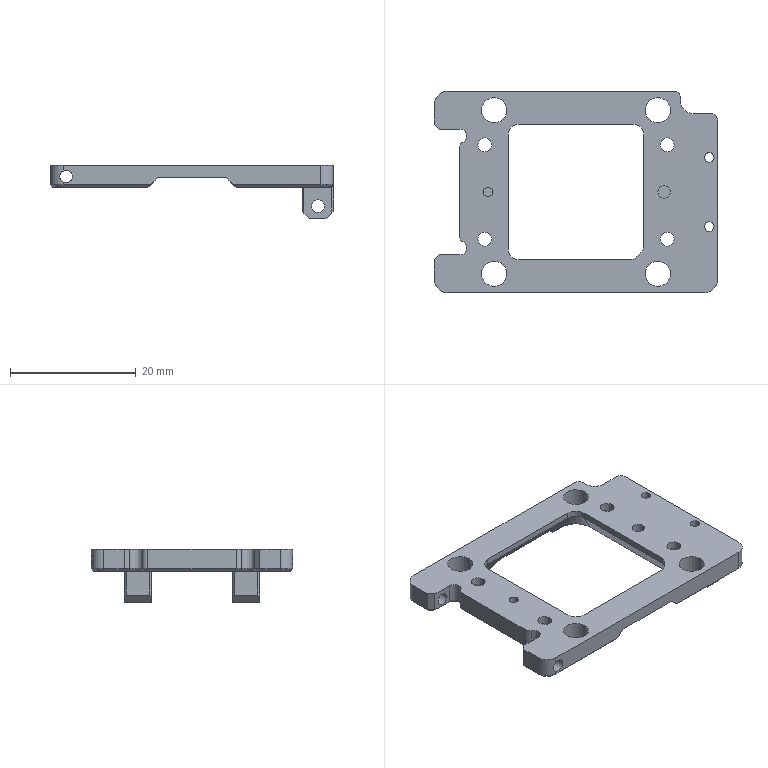NC program | NX | posted with a generic post | part box 45 x 32 x 8.5 mm
Lines 1 to 868 of 3806:
N10 G17 G21 G94 G90
(FLOOR_WALL , TOOL : D63)
N12 T03 M6
N14 G54
N16 G17 G0 G90 X-60. Y-1. B0. C0. S6500 M3
N18 G43 Z30. H3
N20 Z3.
N22 G94 G1 Z0. F1250.
N24 X-57.
N26 X57.
N28 X60.
N30 Z3.
N32 G0 Z30.
N34 M5
(DRILLING , TOOL : D6A45)
N36 T01 M6
N38 G54
N40 G17 G0 G90 X-13. Y13. B0. C0. S5000 M3
N42 G43 Z30. H1
N44 G94 G81 G98 Z-0.6 F250. R3.
N46 X-14.5 Y7.5
N48 X-14. Y0.
N50 X-14.5 Y-7.5
N52 X-13. Y-13.
N54 X13.
N56 X14.5 Y-7.5
N58 X21.2 Y-5.5
N60 X14. Y0.
N62 X21.2 Y5.5
N64 X14.5 Y7.5
N66 X13. Y13.
N68 G80
N70 G0 X13. Y13. Z30.
N72 M5
(DRILLING_COPY_COPY , TOOL : 2.2ZT)
N74 T12 M6
N76 G54
N78 G17 G0 G90 X14.5 Y7.5 B0. C0. S1447 M3
N80 G43 Z30. H12
N82 G94 G83 G98 Z-3.461 F100. Q2. R3.
N84 Y-7.5
N86 X-14.5
N88 Y7.5
N90 G80
N92 G0 X-14.5 Y7.5 Z30.
N94 M5
(DRILLING_COPY_COPY_1 , TOOL : 1.5ZT)
N96 T20 M6
N98 G54
N100 G17 G0 G90 X21.2 Y5.5 B0. C0. S2000 M3
N102 G43 Z30. H20
N104 G94 G83 G98 Z-5.451 F100. Q1. R3.
N106 Y-5.5
N108 G80
N110 G0 X21.2 Y-5.5 Z30.
N112 M5
(DRILLING_COPY_COPY_COPY , TOOL : 4.0ZT)
N114 T09 M6
N116 G54
N118 G17 G0 G90 X13. Y13. B0. C0. S1447 M3
N120 G43 Z30. H9
N122 G94 G83 G98 Z-6.202 F100. Q2. R3.
N124 Y-13.
N126 X-13.
N128 Y13.
N130 G80
N132 G0 X-13. Y13. Z30.
N134 M5
(ADAPTIVE_MILLING , TOOL : D6)
N136 T06 M6
N138 G54
N140 G17 G0 G90 X-30.144 Y-10.787 B0. C0. S9500 M3
N142 G43 Z30. H6
N144 Z-7.5
N146 G94 G1 Z-8.5 F1000.
N148 X-29.181 Y-11.11 F3000.
N150 G3 X-28.537 Y-10.787 R0.611
N152 X-28.017 Y-8.202 R6.628
N154 X-27.907 Y-0.404 R180.736
N156 G2 X-27.878 Y15.57 R931.852
N158 X-25.51 Y18.38 R3.94
N160 X-21.131 Y19.288 R11.792
N162 X-11.833 Y19.393 R240.476
N164 G1 X23.717
N166 X23.792 Y19.392
N168 X23.867 Y19.388
N170 X23.942 Y19.382
N172 X24.017 Y19.374
N174 G2 X26.858 Y17.047 R3.894
N176 X27.794 Y12.524 R11.939
N178 X27.892 Y4.2 R244.742
N180 G1 X27.893 Y-7.725
N182 Y-17.175
N184 X27.892 Y-17.25
N186 X27.89 Y-17.325
N188 X27.885 Y-17.4
N190 X27.878 Y-17.474
N192 G2 X25.646 Y-20.3 R3.826
N194 X21.282 Y-21.263 R11.208
N196 X9.584 Y-21.381 R273.049
N198 G1 X-23.716 Y-21.392
N200 X-23.791 Y-21.391
N202 X-23.866 Y-21.387
N204 X-23.94 Y-21.381
N206 X-24.015 Y-21.374
N208 G2 X-26.857 Y-19.048 R3.893
N210 X-27.79 Y-14.599 R11.787
N212 X-27.584 Y-9.889 R22.068
N214 G3 X-27.317 Y-0.896 R98.508
N216 G1 X-27.314 Y1.579
N218 X-27.312 Y9.004
N220 Y13.354
N222 X-27.309 Y13.504
N224 X-27.301 Y13.653
N226 X-27.289 Y13.803
N228 G2 X-24.364 Y17.613 R4.867
N230 G3 X-23.036 Y18.476 R5.511
N232 G2 X-20.479 Y19.15 R6.035
N234 G1 X15.597
N236 X15.639 Y19.147
N238 G3 X22.125 Y18.8 R44.001
N240 G2 X26.031 Y16.016 R4.79
N242 X27.152 Y11.077 R12.682
N244 X27.285 Y1.854 R189.651
N246 G1 X27.287 Y-6.471
N248 Y-15.321
N250 X27.285 Y-15.471
N252 X27.279 Y-15.621
N254 X27.268 Y-15.77
N256 G2 X24.43 Y-19.558 R4.81
N258 X19.706 Y-20.627 R12.635
N260 X11.159 Y-20.772 R162.134
N262 G1 X6.134 Y-20.776
N264 X-21.841 Y-20.785
N266 X-21.916
N268 X-22.066 Y-20.78
N270 X-22.141 Y-20.776
N272 X-22.291 Y-20.765
N274 G2 X-26.107 Y-17.851 R4.85
N276 X-27.075 Y-11.916 R12.339
N278 G3 X-26.72 Y3.151 R200.631
N280 G2 X-26.68 Y12.525 R294.534
N282 X-25.449 Y15.393 R5.271
N284 X-24.108 Y17.667 R5.815
N286 G1 X-23.87 Y17.85
N288 G3 X-23.636 Y18.321 R0.614
N290 G1 X-23.633 Y18.64
N292 X-23.624 Y19.84 Z-8.4
N294 G2 X-23.172 Y20.458 R0.607
N296 X-20.976 Y20.885 R12.212
N298 G1 X-19.668 Y20.971
N300 X-18.358 Y21.014
N302 X15.308 Y21.35
N304 G2 X15.898 Y20.886 R0.605
N306 G1 X15.957 Y20.634
N308 X16.227 Y19.465 Z-8.5
N310 G3 X16.658 Y19.012 R0.609
N312 X20.024 Y18.321 R9.085
N314 G2 X25.587 Y14.508 R5.788
N316 X26.57 Y9.074 R16.422
N318 X26.679 Y-0.15 R275.392
N320 G1 X26.68 Y-7.8
N322 Y-13.725
N324 X26.678 Y-13.95
N326 X26.676 Y-14.025
N328 X26.667 Y-14.25
N330 X26.656 Y-14.399
N332 G2 X23.298 Y-18.928 R5.473
N334 X18.044 Y-20.03 R14.603
N336 X8.671 Y-20.167 R206.376
N338 G1 X2.446 Y-20.171
N340 X-20.279 Y-20.178
N342 X-20.429 Y-20.176
N344 X-20.579 Y-20.172
N346 X-20.729 Y-20.166
N348 X-20.804 Y-20.162
N350 G2 X-25.394 Y-16.891 R5.458
N352 X-26.346 Y-11.925 R11.302
N354 G3 X-26.112 Y10.797 R716.655
N356 G2 X-25.65 Y13.207 R8.49
N358 X-25.43 Y15.441 R9.186
N360 G3 X-25.434 Y15.909 R0.625
N362 G1 X-25.647 Y16.399
N364 X-26.124 Y17.5 Z-8.4
N366 G2 X-26.129 Y18.049 R0.62
N368 X-25.644 Y18.838 R3.077
N370 G1 X-24.474 Y19.864
N372 G2 X-23.035 Y20.56 R4.205
N374 X-20.895 Y20.94 R13.721
N376 G1 X-19.868 Y21.027
N378 X-18.839 Y21.06
N380 X15.873 Y21.126
N382 G2 X16.487 Y20.564 R0.644
N384 G1 X16.812 Y19.409 Z-8.5
N386 X16.882 Y19.165
N388 X17.005 Y18.944
N390 X17.108 Y18.858
N392 X17.223 Y18.788
N394 G3 X18.553 Y18.184 R32.681
N396 G2 X21.165 Y17.512 R33.868
N398 X24.857 Y13.822 R6.643
N400 X25.68 Y11.433 R4.399
N402 X26.059 Y3.423 R64.029
N404 X26.038 Y-13.301 R759.858
N406 X25.37 Y-15.584 R5.874
N408 X24.108 Y-17.667 R5.525
N410 X21.791 Y-18.98 R5.884
N412 X12.51 Y-19.543 R63.462
N414 G1 X11.31 Y-19.551
N416 X9.811 Y-19.556
N418 X7.486 Y-19.561
N420 X2.161 Y-19.564
N422 X-18.914 Y-19.571
N424 X-19.139 Y-19.569
N426 G2 X-22.097 Y-18.865 R6.159
N428 X-24.167 Y-17.608 R5.507
N430 X-25.48 Y-15.291 R5.884
N432 X-25.69 Y-10.305 R26.123
N434 G3 X-25.525 Y9.942 R789.618
N436 G1 X-25.548 Y10.026
N438 X-25.647 Y10.779
N440 X-25.65 Y10.821
N442 Y13.221
N444 G3 X-26.039 Y13.786 R0.618
N446 G1 X-27.109 Y14.328 Z-8.4
N448 G2 X-27.561 Y14.757 R0.745
N450 G1 X-27.588 Y14.943
N452 X-27.559 Y15.13
N454 G2 X-26.896 Y16.878 R13.154
N456 X-25.822 Y18.586 R8.756
N458 X-22.937 Y20.573 R6.783
N460 X-20.073 Y21.13 R7.715
N462 G1 X13.95 Y21.123
N464 G2 X16.48 Y20.881 R24.277
N466 X16.878 Y20.519 R0.613
N468 G1 X17.317 Y19.403 Z-8.5
N470 X17.583 Y18.743
N472 X17.739 Y18.561
N474 G3 X19.968 Y17.353 R7.024
N476 G2 X22.834 Y15.35 R8.241
N478 X24.871 Y13.803 R4.032
N480 G3 X25.76 Y14.755 R-0.66
N482 G1 X23.431 Y16.302
N484 X22.431 Y16.966 Z-8.4
N486 X19.892 Y18.654
N488 X18.964 Y19.263 Z-8.492
N490 X18.88 Y19.297 Z-8.5
N492 G3 X18.273 Y18.147 R0.66
N494 X20.687 Y16.306 R28.606
N496 X21.736 Y15.556 R4.244
N498 G2 X22.959 Y15.286 R3.477
N500 G3 X23.756 Y16.27 R0.66
N502 X23.299 Y16.609 Z-8.452 R1.319
N504 G1 X22.759 Y16.924 Z-8.4
N506 X19.973 Y18.55
N508 X19.651 Y18.742 Z-8.431
N510 X19.316 Y18.911 Z-8.463
N512 G3 X18.877 Y18.896 Z-8.5 R0.679
N514 X18.594 Y17.885 R0.662
N516 X20.854 Y15.619 R7.438
N518 G1 X20.926 Y15.6
N520 X21.003 Y15.587
N522 X21.479
N524 X21.521 Y15.585
N526 X21.744 Y15.555
N528 G3 X22.186 Y16.765 R0.66
N530 G1 X21.037 Y17.506
N532 X19.878 Y18.232
N534 G3 X19.092 Y17.227 R0.66
N536 X19.718 Y16.163 R27.834
N538 X21.026 Y15.587 R1.251
N540 X21.417 Y16.779 R0.66
N542 G1 X20.24 Y17.636
N544 G3 X19.327 Y16.801 R0.661
N546 X19.872 Y15.742 R3.008
N548 X20.548 Y15.587 R1.151
N550 X20.839 Y16.839 R0.66
N552 G1 X20.385 Y17.054
N554 G3 X19.58 Y16.175 R0.661
N556 G1 X19.612 Y16.096
N558 X19.671 Y15.984
N560 X19.73 Y15.895
N562 X19.781 Y15.84
N564 G3 X20.116 Y15.622 R0.673
N566 G1 X20.323 Y15.587
N568 X21.521 Y15.585
N570 X22.068 Y15.518
N572 X22.613 Y15.43
N574 X23.114 Y15.227
N576 X23.608 Y15.006
N578 X24.04 Y14.68
N580 X24.46 Y14.339
N582 X24.793 Y13.912
N584 X25.11 Y13.474
N586 X25.322 Y12.976
N588 X25.514 Y12.47
N590 X25.647 Y11.458
N592 X25.65 Y11.416
N594 Y-13.979
N596 X25.647 Y-14.021
N598 X25.48 Y-15.291
N600 X25.459 Y-15.372
N602 X25.344 Y-15.649
N604 X25.148 Y-16.132
N606 X24.935 Y-16.608
N608 X24.531 Y-17.145
N610 X24.108 Y-17.667
N612 X23.58 Y-18.081
N614 X23.036 Y-18.476
N616 X22.418 Y-18.739
N618 X21.791 Y-18.98
N620 X20.521 Y-19.147
N622 X20.479 Y-19.15
N624 X-20.479
N626 X-20.521 Y-19.147
N628 X-21.791 Y-18.98
N630 X-21.872 Y-18.959
N632 X-22.149 Y-18.844
N634 X-22.632 Y-18.648
N636 X-23.108 Y-18.435
N638 X-23.645 Y-18.031
N640 X-24.167 Y-17.608
N642 X-24.581 Y-17.08
N644 X-24.976 Y-16.536
N646 X-25.239 Y-15.918
N648 X-25.48 Y-15.291
N650 X-25.65 Y-13.979
N652 Y-10.821
N654 X-25.647 Y-10.779
N656 G2 X-25.297 Y-9. R14.745
N658 G3 X-24.966 Y-2.563 R49.993
N660 G1 X-24.954 Y-1.213
N662 X-24.944 Y0.212
N664 X-24.939 Y1.637
N666 X-24.936 Y2.837
N668 X-24.933 Y3.512
N670 X-24.931 Y4.562
N672 Y5.387
N674 X-24.928 Y6.137
N676 Y6.737
N678 X-24.925 Y7.487
N680 X-24.92 Y8.237
N682 Y8.461
N684 X-24.923 Y8.611
N686 X-24.929 Y8.686
N688 X-24.943 Y8.76
N690 G3 X-25.244 Y9.264 R3.63
N692 G1 X-25.527 Y9.946
N694 G3 X-26.517 Y10.233 R0.662
N696 X-26.796 Y9.58 Z-8.438 R0.712
N698 G1 Y9.124 Z-8.4
N700 Y-9.084
N702 X-26.8 Y-9.462 Z-8.432
N704 X-26.778 Y-9.84 Z-8.463
N706 G3 X-26.549 Y-10.209 Z-8.5 R0.681
N708 X-25.527 Y-9.946 R0.662
N710 X-24.532 Y-5.98 R9.59
N712 X-24.333 Y5.191 R192.621
N714 X-24.398 Y8.112 R22.651
N716 X-24.74 Y8.589 R1.366
N718 G1 X-25.06 Y9.006
N720 G3 X-25.902 Y9.182 R0.664
N722 X-26.244 Y8.498 Z-8.433 R0.702
N724 G1 X-26.247 Y8.108 Z-8.4
N726 X-26.382 Y-8.264
N728 X-26.387 Y-8.597 Z-8.428
N730 X-26.37 Y-8.929 Z-8.456
N732 G3 X-26.071 Y-9.353 Z-8.5 R0.668
N734 X-25.203 Y-9.192 R0.664
N736 X-24.136 Y-6.512 R5.083
N738 X-23.774 Y-0.003 R48.227
N740 X-23.792 Y7.195 R108.609
N742 X-23.993 Y7.838 R1.451
N744 G1 X-24.576 Y8.421
N746 G3 X-25.367 Y8.53 R0.665
N748 X-25.705 Y7.855 Z-8.434 R0.705
N750 G1 X-25.714 Y7.453 Z-8.4
N752 X-26.055 Y-7.829
N754 X-26.065 Y-8.165 Z-8.428
N756 X-26.052 Y-8.501 Z-8.456
N758 G3 X-25.767 Y-8.926 Z-8.5 R0.669
N760 X-24.883 Y-8.775 R0.664
N762 X-23.642 Y-6.123 R4.829
N764 X-23.194 Y0.003 R37.335
N766 X-23.204 Y6.451 R93.375
N768 X-23.549 Y7.499 R1.644
N770 G1 X-23.907 Y7.758
N772 X-23.945 Y7.791
N774 X-23.998 Y7.844
N776 G3 X-24.779 Y7.958 R0.665
N778 X-25.129 Y7.288 Z-8.434 R0.705
N780 G1 X-25.145 Y6.888 Z-8.4
N782 X-25.712 Y-7.426
N784 X-25.728 Y-7.763 Z-8.428
N786 X-25.721 Y-8.101 Z-8.456
N788 G3 X-25.446 Y-8.53 Z-8.5 R0.669
N790 X-24.607 Y-8.452 R0.664
N792 X-23.156 Y-5.807 R4.552
N794 X-22.618 Y0.083 R30.621
N796 X-22.636 Y5.93 R60.554
N798 X-23.019 Y7.122 R1.986
N800 G1 X-23.077 Y7.169
N802 X-23.111 Y7.193
N804 X-23.157 Y7.216
N806 X-23.583 Y7.524
N808 G3 X-24.311 Y7.553 R0.666
N810 X-24.634 Y6.907 Z-8.437 R0.707
N812 G1 X-24.653 Y6.467 Z-8.4
N814 X-25.232 Y-6.941
N816 X-25.249 Y-7.28 Z-8.428
N818 X-25.245 Y-7.62 Z-8.457
N820 G3 X-24.975 Y-8.048 Z-8.5 R0.67
N822 X-24.129 Y-7.974 R0.664
N824 X-22.666 Y-5.498 R4.261
N826 X-22.042 Y0.307 R27.072
N828 X-22.103 Y5.701 R36.776
N830 X-22.626 Y6.995 R2.077
N832 G1 X-22.689 Y7.036
N834 X-22.766 Y7.076
N836 X-23.067 Y7.171
N838 X-23.134 Y7.205
N840 G3 X-23.774 Y7.179 R0.67
N842 X-24.097 Y6.541 Z-8.438 R0.71
N844 G1 X-24.123 Y6.092 Z-8.4
N846 X-24.86 Y-6.592
N848 X-24.885 Y-6.947 Z-8.43
N850 X-24.879 Y-7.302 Z-8.459
N852 G3 X-24.628 Y-7.707 Z-8.5 R0.672
N854 X-23.846 Y-7.714 R0.665
N856 X-22.22 Y-5.368 R3.844
N858 X-21.65 Y-2.299 R16.994
N860 X-21.681 Y5.5 R315.492
N862 X-22.216 Y6.865 R2.088
N864 G1 X-22.783 Y7.081
N866 G3 X-23.577 Y6.166 R0.661
N868 G1 X-22.853 Y4.675
N870 G3 X-21.65 Y5.051 R0.66
N872 X-21.761 Y6.535 R4.031
N874 X-22.365 Y6.948 R0.954
N876 X-23.063 Y5.887 R0.66
N878 G1 X-22.87 Y5.658
N880 X-22.646 Y5.457
N882 G3 X-21.65 Y6.026 R0.661
N884 X-21.941 Y6.753 R0.822
N886 X-22.982 Y6.29 R0.661
N888 G1 X-23.014 Y6.002
N890 X-23.149 Y4.81 Z-8.4
N892 X-24.401 Y-6.253
N894 X-24.446 Y-6.605 Z-8.43
N896 X-24.459 Y-6.959 Z-8.459
N898 G3 X-24.23 Y-7.378 Z-8.5 R0.672
N900 X-23.42 Y-7.406 R0.665
N902 X-21.77 Y-5.23 R3.687
N904 G1 X-21.721 Y-5.088
N906 X-21.674 Y-4.946
N908 X-21.657 Y-4.873
N910 X-21.65 Y-4.821
N912 Y-2.271
N914 G3 X-22.773 Y-1.8 R0.661
N916 X-22.994 Y-2.285 Z-8.455 R0.909
N918 G1 X-23.153 Y-2.924 Z-8.4
N920 X-23.894 Y-5.898
N922 X-23.985 Y-6.243 Z-8.43
N924 X-24.045 Y-6.594 Z-8.46
N926 G3 X-23.875 Y-7.037 Z-8.5 R0.673
N928 X-23.09 Y-7.182 R0.665
N930 X-21.65 Y-5.695 R2.302
N932 G1 Y-4.795
N934 G3 X-22.905 Y-4.51 R0.66
N936 G1 X-23.758 Y-6.314
N938 G3 X-22.924 Y-7.126 R0.661
N940 X-21.681 Y-6.254 R1.713
N942 G1 X-21.662 Y-6.181
N944 X-21.65 Y-6.107
N946 Y-5.657
N948 G3 X-22.869 Y-5.306 R0.66
N950 G1 X-23.374 Y-6.127
N952 G3 X-22.567 Y-7.012 R0.661
N954 X-21.69 Y-6.399 R1.092
N956 G1 X-21.66 Y-6.289
N958 X-21.65 Y-6.176
N960 Y-6.101
N962 G3 X-22.297 Y-5.497 R0.609
N964 G1 X-23.159 Y-5.555
N966 Z-5.5
N968 G0 Z30.
N970 X2.147 Y-1.637
N972 Z1.
N974 G3 X2.147 Y-1.637 Z0.763 I-2.147 J1.637 F1000.
N976 X2.147 Y-1.637 Z0.526 I-2.147 J1.637
N978 X2.147 Y-1.637 Z0.289 I-2.147 J1.637
N980 X2.147 Y-1.637 Z0.052 I-2.147 J1.637
N982 X2.147 Y-1.637 Z-0.184 I-2.147 J1.637
N984 X2.147 Y-1.637 Z-0.421 I-2.147 J1.637
N986 X2.147 Y-1.637 Z-0.658 I-2.147 J1.637
N988 X2.147 Y-1.637 Z-0.895 I-2.147 J1.637
N990 X2.147 Y-1.637 Z-1.132 I-2.147 J1.637
N992 X2.147 Y-1.637 Z-1.369 I-2.147 J1.637
N994 X2.147 Y-1.637 Z-1.606 I-2.147 J1.637
N996 X2.147 Y-1.637 Z-1.843 I-2.147 J1.637
N998 X2.147 Y-1.637 Z-2.08 I-2.147 J1.637
N1000 X2.147 Y-1.637 Z-2.316 I-2.147 J1.637
N1002 X2.147 Y-1.637 Z-2.553 I-2.147 J1.637
N1004 X2.147 Y-1.637 Z-2.79 I-2.147 J1.637
N1006 X2.147 Y-1.637 Z-3.027 I-2.147 J1.637
N1008 X2.147 Y-1.637 Z-3.264 I-2.147 J1.637
N1010 X2.147 Y-1.637 Z-3.501 I-2.147 J1.637
N1012 X2.147 Y-1.637 Z-3.738 I-2.147 J1.637
N1014 X2.147 Y-1.637 Z-3.975 I-2.147 J1.637
N1016 X2.147 Y-1.637 Z-4.211 I-2.147 J1.637
N1018 X2.147 Y-1.637 Z-4.448 I-2.147 J1.637
N1020 X2.147 Y-1.637 Z-4.685 I-2.147 J1.637
N1022 X2.147 Y-1.637 Z-4.922 I-2.147 J1.637
N1024 X2.147 Y-1.637 Z-5.159 I-2.147 J1.637
N1026 X2.147 Y-1.637 Z-5.396 I-2.147 J1.637
N1028 X2.147 Y-1.637 Z-5.633 I-2.147 J1.637
N1030 X2.147 Y-1.637 Z-5.87 I-2.147 J1.637
N1032 X2.147 Y-1.637 Z-6.107 I-2.147 J1.637
N1034 X2.147 Y-1.637 Z-6.343 I-2.147 J1.637
N1036 X2.147 Y-1.637 Z-6.58 I-2.147 J1.637
N1038 X2.147 Y-1.637 Z-6.817 I-2.147 J1.637
N1040 X2.147 Y-1.637 Z-7.054 I-2.147 J1.637
N1042 X2.147 Y-1.637 Z-7.291 I-2.147 J1.637
N1044 X2.147 Y-1.637 Z-7.528 I-2.147 J1.637
N1046 X2.147 Y-1.637 Z-7.765 I-2.147 J1.637
N1048 X2.147 Y-1.637 Z-8.002 I-2.147 J1.637
N1050 X2.147 Y-1.637 Z-8.239 I-2.147 J1.637
N1052 X2.147 Y-1.637 Z-8.475 I-2.147 J1.637
N1054 X2.7 Y0. Z-8.5 R2.7
N1056 X2.23 Y-1.533 R-2.701 F3000.
N1058 X-1.402 Y2.621 R2.814
N1060 X2.454 Y-1.726 R-2.982
N1062 X-1.832 Y2.7 R3.116
N1064 X2.739 Y-1.845 R-3.277
N1066 X-2.145 Y2.845 R3.42
N1068 X2.933 Y-2.099 R-3.58
N1070 X-2.753 Y2.726 R3.735
N1072 X3.023 Y-2.5 R-3.897
N1074 X-3.048 Y2.888 R4.059
N1076 X3.174 Y-2.829 R-4.225
N1078 X-3.229 Y3.183 R4.392
N1080 X3.408 Y-3.082 R-4.564
N1082 X3.171 Y3.614 R4.738
N1084 X-3.507 Y3.396 R4.738
N1086 X3.523 Y-3.469 R4.913
N1088 X-3.43 Y3.963 R5.09
N1090 X3.737 Y-3.769 R-5.273
N1092 X-3.937 Y3.99 R-5.457
N1094 X3.826 Y-4.194 R5.642
N1096 X-4.092 Y4.365 R-5.831
N1098 X4.296 Y-4.276 R-6.022
N1100 X-4.117 Y4.857 R6.212
N1102 X4.403 Y-4.707 R-6.406
N1104 X-4.287 Y5.232 R6.603
N1106 X4.929 Y-4.752 R-6.803
N1108 X-4.624 Y5.466 R7.
N1110 X4.522 Y-5.653 R7.2
N1112 X-4.559 Y6.036 R7.401
N1114 X4.548 Y-6.143 R7.605
N1116 G1 X4.859 Y-5.906
N1118 X5.156 Y-5.651
N1120 G3 X7.65 Y-1.354 R7.546
N1122 X7.569 Y1.791 R22.751
N1124 X2.157 Y7.65 R7.586
N1126 X-1.966 Y7.608 R63.988
N1128 X-7.65 Y2.362 R7.395
N1130 X-7.614 Y-1.986 R90.953
N1132 X-3.104 Y-7.404 R7.349
N1134 G1 X-2.966 Y-7.462
N1136 X-2.826 Y-7.516
N1138 X-2.685 Y-7.568
N1140 X-2.543 Y-7.617
N1142 X-2.471 Y-7.637
N1144 X-2.391 Y-7.65
N1146 G3 X2.182 Y-7.603 R59.161
N1148 X7.65 Y-2.836 R7.45
N1150 G1 Y0.971
N1152 G3 X7.458 Y3.35 R7.377
N1154 X3.412 Y7.642 R7.35
N1156 G1 X3.358 Y7.65
N1158 X2.083
N1160 G3 X1.438 Y7.133 R0.664
N1162 X1.712 Y6.432 Z-8.434 R0.707
N1164 G1 X2.006 Y6.152 Z-8.4
N1166 X6.135 Y2.223
N1168 X6.39 Y1.974 Z-8.43
N1170 X6.666 Y1.748 Z-8.46
N1172 G3 X7.135 Y1.677 Z-8.5 R0.673
N1174 X7.65 Y2.321 R0.664
N1176 X6.245 Y6.141 R4.858
N1178 X4.38 Y7.627 R6.702
N1180 G1 X4.307 Y7.643
N1182 X4.259 Y7.65
N1184 X3.284
N1186 G3 X2.643 Y7.148 R0.665
N1188 X2.895 Y6.444 Z-8.434 R0.708
N1190 G1 X3.183 Y6.151 Z-8.4
N1192 X6.137 Y3.147
N1194 X6.382 Y2.891 Z-8.43
N1196 X6.648 Y2.658 Z-8.459
N1198 G3 X7.119 Y2.573 Z-8.5 R0.672
N1200 X7.65 Y3.221 R0.664
N1202 X6.356 Y6.615 R4.303
N1204 X5.082 Y7.637 R3.503
N1206 G1 X5.002 Y7.65
N1208 X4.252
N1210 G3 X3.616 Y7.167 R0.665
N1212 X3.843 Y6.459 Z-8.435 R0.71
N1214 G1 X4.122 Y6.15 Z-8.4
N1216 X6.138 Y3.927
N1218 X6.365 Y3.673 Z-8.428
N1220 X6.608 Y3.435 Z-8.457
N1222 G3 X7.099 Y3.32 Z-8.5 R0.67
N1224 X7.65 Y3.971 R0.664
N1226 X6.395 Y7.141 R3.951
N1228 X5.619 Y7.65 R1.448
N1230 G1 X4.944
N1232 G3 X4.447 Y6.556 R0.661
N1234 G1 X5.502 Y5.341
N1236 X6.569 Y4.137
N1238 G3 X7.65 Y4.646 R0.661
N1240 X6.347 Y7.59 R3.226
N1242 X5.6 Y7.65 R2.473
N1244 X5.093 Y6.568 R0.661
N1246 G1 X6.558 Y4.822
N1248 G3 X7.65 Y5.321 R0.661
N1250 X6.828 Y7.549 R2.584
N1252 X6.079 Y7.65 R1.496
N1254 X5.576 Y6.562 R0.661
N1256 G1 X6.563 Y5.417
N1258 G3 X7.65 Y5.921 R0.661
N1260 X7.169 Y7.512 R1.939
N1262 X6.516 Y7.65 R1.052
N1264 X6.018 Y6.557 R0.661
N1266 G1 X6.568 Y5.938
N1268 G3 X7.65 Y6.446 R0.661
N1270 X7.324 Y7.521 R1.177
N1272 X6.773 Y7.65 R1.07
N1274 X6.367 Y6.47 R0.661
N1276 G1 X6.557 Y6.32
N1278 X6.767 Y6.199
N1280 G3 X7.65 Y6.821 R0.662
N1282 X7.31 Y7.53 R0.777
N1284 X6.46 Y7.251 R0.602
N1286 G1 X6.409 Y7. Z-8.479
N1288 X6.408 Y6.745 Z-8.457
N1290 G2 X6.146 Y6.145 Z-8.4 R0.648
N1292 G1 X5.983 Y6.069
N1294 X5.805 Y6.041
N1296 X-0.334 Y6.076
N1298 X-0.499 Y6.126
N1300 G2 X-0.844 Y6.779 Z-8.466 R0.637
N1302 G1 X-0.859 Y7.188 Z-8.5
N1304 G3 X-1.443 Y7.65 R0.605
N1306 X-3.945 Y7.319 R5.644
N1308 X-7.644 Y3.561 R7.22
N1310 G1 X-7.65 Y3.517
N1312 Y2.317
N1314 G3 X-7.131 Y1.672 R0.664
N1316 X-6.431 Y1.948 Z-8.434 R0.707
N1318 G1 X-6.152 Y2.242 Z-8.4
N1320 X-2.468 Y6.135
N1322 X-2.22 Y6.391 Z-8.43
N1324 X-1.994 Y6.667 Z-8.46
N1326 G3 X-1.924 Y7.136 Z-8.5 R0.673
N1328 X-2.568 Y7.65 R0.665
N1330 X-6.126 Y6.367 R4.554
N1332 X-7.628 Y4.517 R6.411
N1334 G1 X-7.644 Y4.443
N1336 X-7.65 Y4.398
N1338 Y3.498
N1340 G3 X-7.151 Y2.858 R0.665
N1342 X-6.446 Y3.106 Z-8.434 R0.708
N1344 G1 X-6.151 Y3.393 Z-8.4
N1346 X-3.324 Y6.137
N1348 X-3.067 Y6.38 Z-8.43
N1350 X-2.833 Y6.645 Z-8.459
N1352 G3 X-2.745 Y7.116 Z-8.5 R0.672
N1354 X-3.393 Y7.65 R0.664
N1356 X-6.6 Y6.469 R4.09
N1358 X-7.636 Y5.207 R3.43
N1360 G1 X-7.65 Y5.122
N1362 Y4.372
N1364 G3 X-6.543 Y3.886 R0.661
N1366 G1 X-5.078 Y5.228
N1368 X-3.624 Y6.581
N1370 G3 X-4.143 Y7.65 R0.661
N1372 X-7.598 Y5.926 R3.822
N1374 X-7.65 Y5.116 R3.258
N1376 X-6.559 Y4.616 R0.661
N1378 G1 X-5.43 Y5.585
N1380 X-4.312 Y6.566
N1382 G3 X-4.818 Y7.65 R0.661
N1384 X-7.609 Y6.383 R2.9
N1386 X-7.65 Y5.683 R4.959
N1388 X-6.568 Y5.176 R0.661
N1390 G1 X-4.919 Y6.558
N1392 G3 X-5.418 Y7.65 R0.661
N1394 X-7.569 Y6.853 R2.398
N1396 X-7.65 Y6.133 R1.735
N1398 X-6.554 Y5.638 R0.661
N1400 G1 X-5.508 Y6.571
N1402 G3 X-6.018 Y7.65 R0.661
N1404 X-7.532 Y7.182 R1.78
N1406 X-7.65 Y6.552 R1.136
N1408 X-6.528 Y6.081 R0.661
N1410 G1 X-6.013 Y6.597
N1412 G3 X-6.543 Y7.65 R0.661
N1414 X-7.492 Y7.375 R1.096
N1416 X-7.65 Y6.848 R1.119
N1418 X-6.187 Y7.129 R-0.756
N1420 X-7.216 Y7.578 R0.756
N1422 X-7.197 Y6.497 R0.601
N1424 G1 X-6.944 Y6.442 Z-8.478
N1426 X-6.685 Y6.439 Z-8.457
N1428 G2 X-6.091 Y6.178 Z-8.4 R0.649
N1430 G1 X-6.013 Y6.012
N1432 X-5.985 Y5.83
N1434 X-6.069 Y-0.442
N1436 X-6.127 Y-0.616
N1438 G2 X-6.775 Y-0.941 Z-8.464 R0.639
N1440 G1 X-6.988 Y-0.939 Z-8.482
N1442 X-7.201 Y-0.957 Z-8.5
N1444 G3 X-7.65 Y-1.538 R0.605
N1446 X-6.048 Y-5.895 R5.353
N1448 X-3.631 Y-7.635 R7.775
N1450 G1 X-3.544 Y-7.65
N1452 X-2.344
N1454 G3 X-1.699 Y-7.127 R0.664
N1456 X-1.979 Y-6.428 Z-8.434 R0.706
N1458 G1 X-2.275 Y-6.152 Z-8.4
N1460 X-6.135 Y-2.557
N1462 X-6.393 Y-2.31 Z-8.43
N1464 X-6.672 Y-2.087 Z-8.46
N1466 G3 X-7.14 Y-2.02 Z-8.5 R0.673
N1468 X-7.65 Y-2.663 R0.665
N1470 X-6.37 Y-6.144 R4.462
N1472 X-4.512 Y-7.634 R5.737
N1474 G1 X-4.439 Y-7.648
N1476 X-4.421 Y-7.65
N1478 X-3.521
N1480 G3 X-2.88 Y-7.146 R0.665
N1482 X-3.135 Y-6.442 Z-8.434 R0.708
N1484 G1 X-3.423 Y-6.151 Z-8.4
N1486 X-6.137 Y-3.411
N1488 X-6.383 Y-3.156 Z-8.43
N1490 X-6.65 Y-2.924 Z-8.459
N1492 G3 X-7.122 Y-2.841 Z-8.5 R0.672
N1494 X-7.65 Y-3.488 R0.664
N1496 X-6.421 Y-6.675 R4.08
N1498 X-5.201 Y-7.641 R3.041
N1500 G1 X-5.135 Y-7.65
N1502 X-4.385
N1504 G3 X-3.9 Y-6.543 R0.661
N1506 G1 X-5.235 Y-5.088
N1508 X-6.582 Y-3.644
N1510 G3 X-7.65 Y-4.163 R0.661
N1512 X-5.918 Y-7.607 R3.761
N1514 X-5.061 Y-7.65 R4.471
N1516 X-4.569 Y-6.549 R0.661
N1518 G1 X-6.575 Y-4.324
N1520 G3 X-7.65 Y-4.838 R0.661
N1522 X-6.443 Y-7.59 R3.014
N1524 X-5.695 Y-7.65 R2.436
N1526 X-5.188 Y-6.567 R0.661
N1528 G1 X-6.559 Y-4.938
N1530 G3 X-7.65 Y-5.438 R0.661
N1532 X-6.907 Y-7.542 R2.446
N1534 X-6.146 Y-7.65 R1.442
N1536 X-5.652 Y-6.552 R0.661
N1538 G1 X-6.573 Y-5.527
N1540 G3 X-7.65 Y-6.038 R0.661
N1542 X-7.171 Y-7.543 R1.718
N1544 X-6.562 Y-7.65 R1.199
N1546 X-6.096 Y-6.523 R0.661
N1548 G1 X-6.602 Y-6.029
N1550 G3 X-7.65 Y-6.563 R0.661
N1552 X-7.23 Y-7.575 R0.939
N1554 G1 X-6.848 Y-7.65
N1556 G3 X-7.129 Y-6.187 R-0.756
N1558 X-7.578 Y-7.216 R0.756
N1560 X-6.497 Y-7.196 R0.601
N1562 G1 X-6.442 Y-6.944 Z-8.478
N1564 X-6.439 Y-6.685 Z-8.457
N1566 G2 X-6.178 Y-6.091 Z-8.4 R0.649
N1568 G1 X-6.012 Y-6.013
N1570 X-5.83 Y-5.985
N1572 X0.563 Y-6.069
N1574 X0.738 Y-6.127
N1576 G2 X1.063 Y-6.775 Z-8.464 R0.638
N1578 G1 X1.061 Y-6.988 Z-8.482
N1580 X1.079 Y-7.201 Z-8.5
N1582 G3 X1.659 Y-7.65 R0.605
N1584 X5.91 Y-6.149 R5.383
N1586 X7.637 Y-3.911 R6.767
N1588 G1 X7.65 Y-3.832
N1590 Y-2.782
N1592 G3 X7.149 Y-2.142 R0.665
N1594 X6.444 Y-2.394 Z-8.434 R0.708
N1596 G1 X6.152 Y-2.681 Z-8.4
N1598 X2.636 Y-6.136
N1600 X2.381 Y-6.381 Z-8.43
N1602 X2.147 Y-6.648 Z-8.459
N1604 G3 X2.062 Y-7.119 Z-8.5 R0.672
N1606 X2.709 Y-7.65 R0.664
N1608 X6.385 Y-6.275 R4.652
N1610 X7.639 Y-4.709 R4.372
N1612 G1 X7.65 Y-4.635
N1614 Y-3.81
N1616 G3 X7.164 Y-3.173 R0.665
N1618 X6.456 Y-3.404 Z-8.435 R0.71
N1620 G1 X6.151 Y-3.685 Z-8.4
N1622 X3.486 Y-6.138
N1624 X3.223 Y-6.373 Z-8.429
N1626 X2.983 Y-6.631 Z-8.459
N1628 G3 X2.884 Y-7.102 Z-8.5 R0.672
N1630 X3.534 Y-7.65 R0.664
N1632 X6.747 Y-6.482 R4.119
N1634 X7.637 Y-5.391 R2.752
N1636 G1 X7.65 Y-5.311
N1638 Y-4.561
N1640 G3 X6.549 Y-4.07 R0.661
N1642 G1 X5.154 Y-5.317
N1644 X3.771 Y-6.576
N1646 G3 X4.284 Y-7.65 R0.661
N1648 X7.589 Y-6.097 R3.667
N1650 X7.65 Y-5.273 R2.637
N1652 X6.564 Y-4.769 R0.661
N1654 G1 X5.506 Y-5.659
N1656 X4.457 Y-6.562
N1658 G3 X4.959 Y-7.65 R0.661
N1660 X7.595 Y-6.542 R2.835
N1662 X7.65 Y-5.799 R2.779
N1664 X6.568 Y-5.292 R0.661
N1666 G1 X5.06 Y-6.558
N1668 G3 X5.559 Y-7.65 R0.661
N1670 X7.54 Y-6.99 R2.317
N1672 X7.65 Y-6.302 R1.295
N1674 X6.569 Y-5.794 R0.661
N1676 G1 X5.661 Y-6.557
N1678 G3 X6.159 Y-7.65 R0.661
N1680 X7.491 Y-7.294 R1.692
N1682 X7.65 Y-6.613 R0.99
N1684 X6.526 Y-6.144 R0.661
N1686 G1 X6.077 Y-6.6
N1688 G3 X6.609 Y-7.65 R0.661
N1690 X7.638 Y-7.048 R0.861
N1692 G1 X7.65 Y-6.923
N1694 Y-6.848
N1696 G3 X7.202 Y-6.263 R0.611
N1698 G1 X6.139 Y-5.975
N1700 Z-5.5
N1702 G0 Z30.
N1704 M5